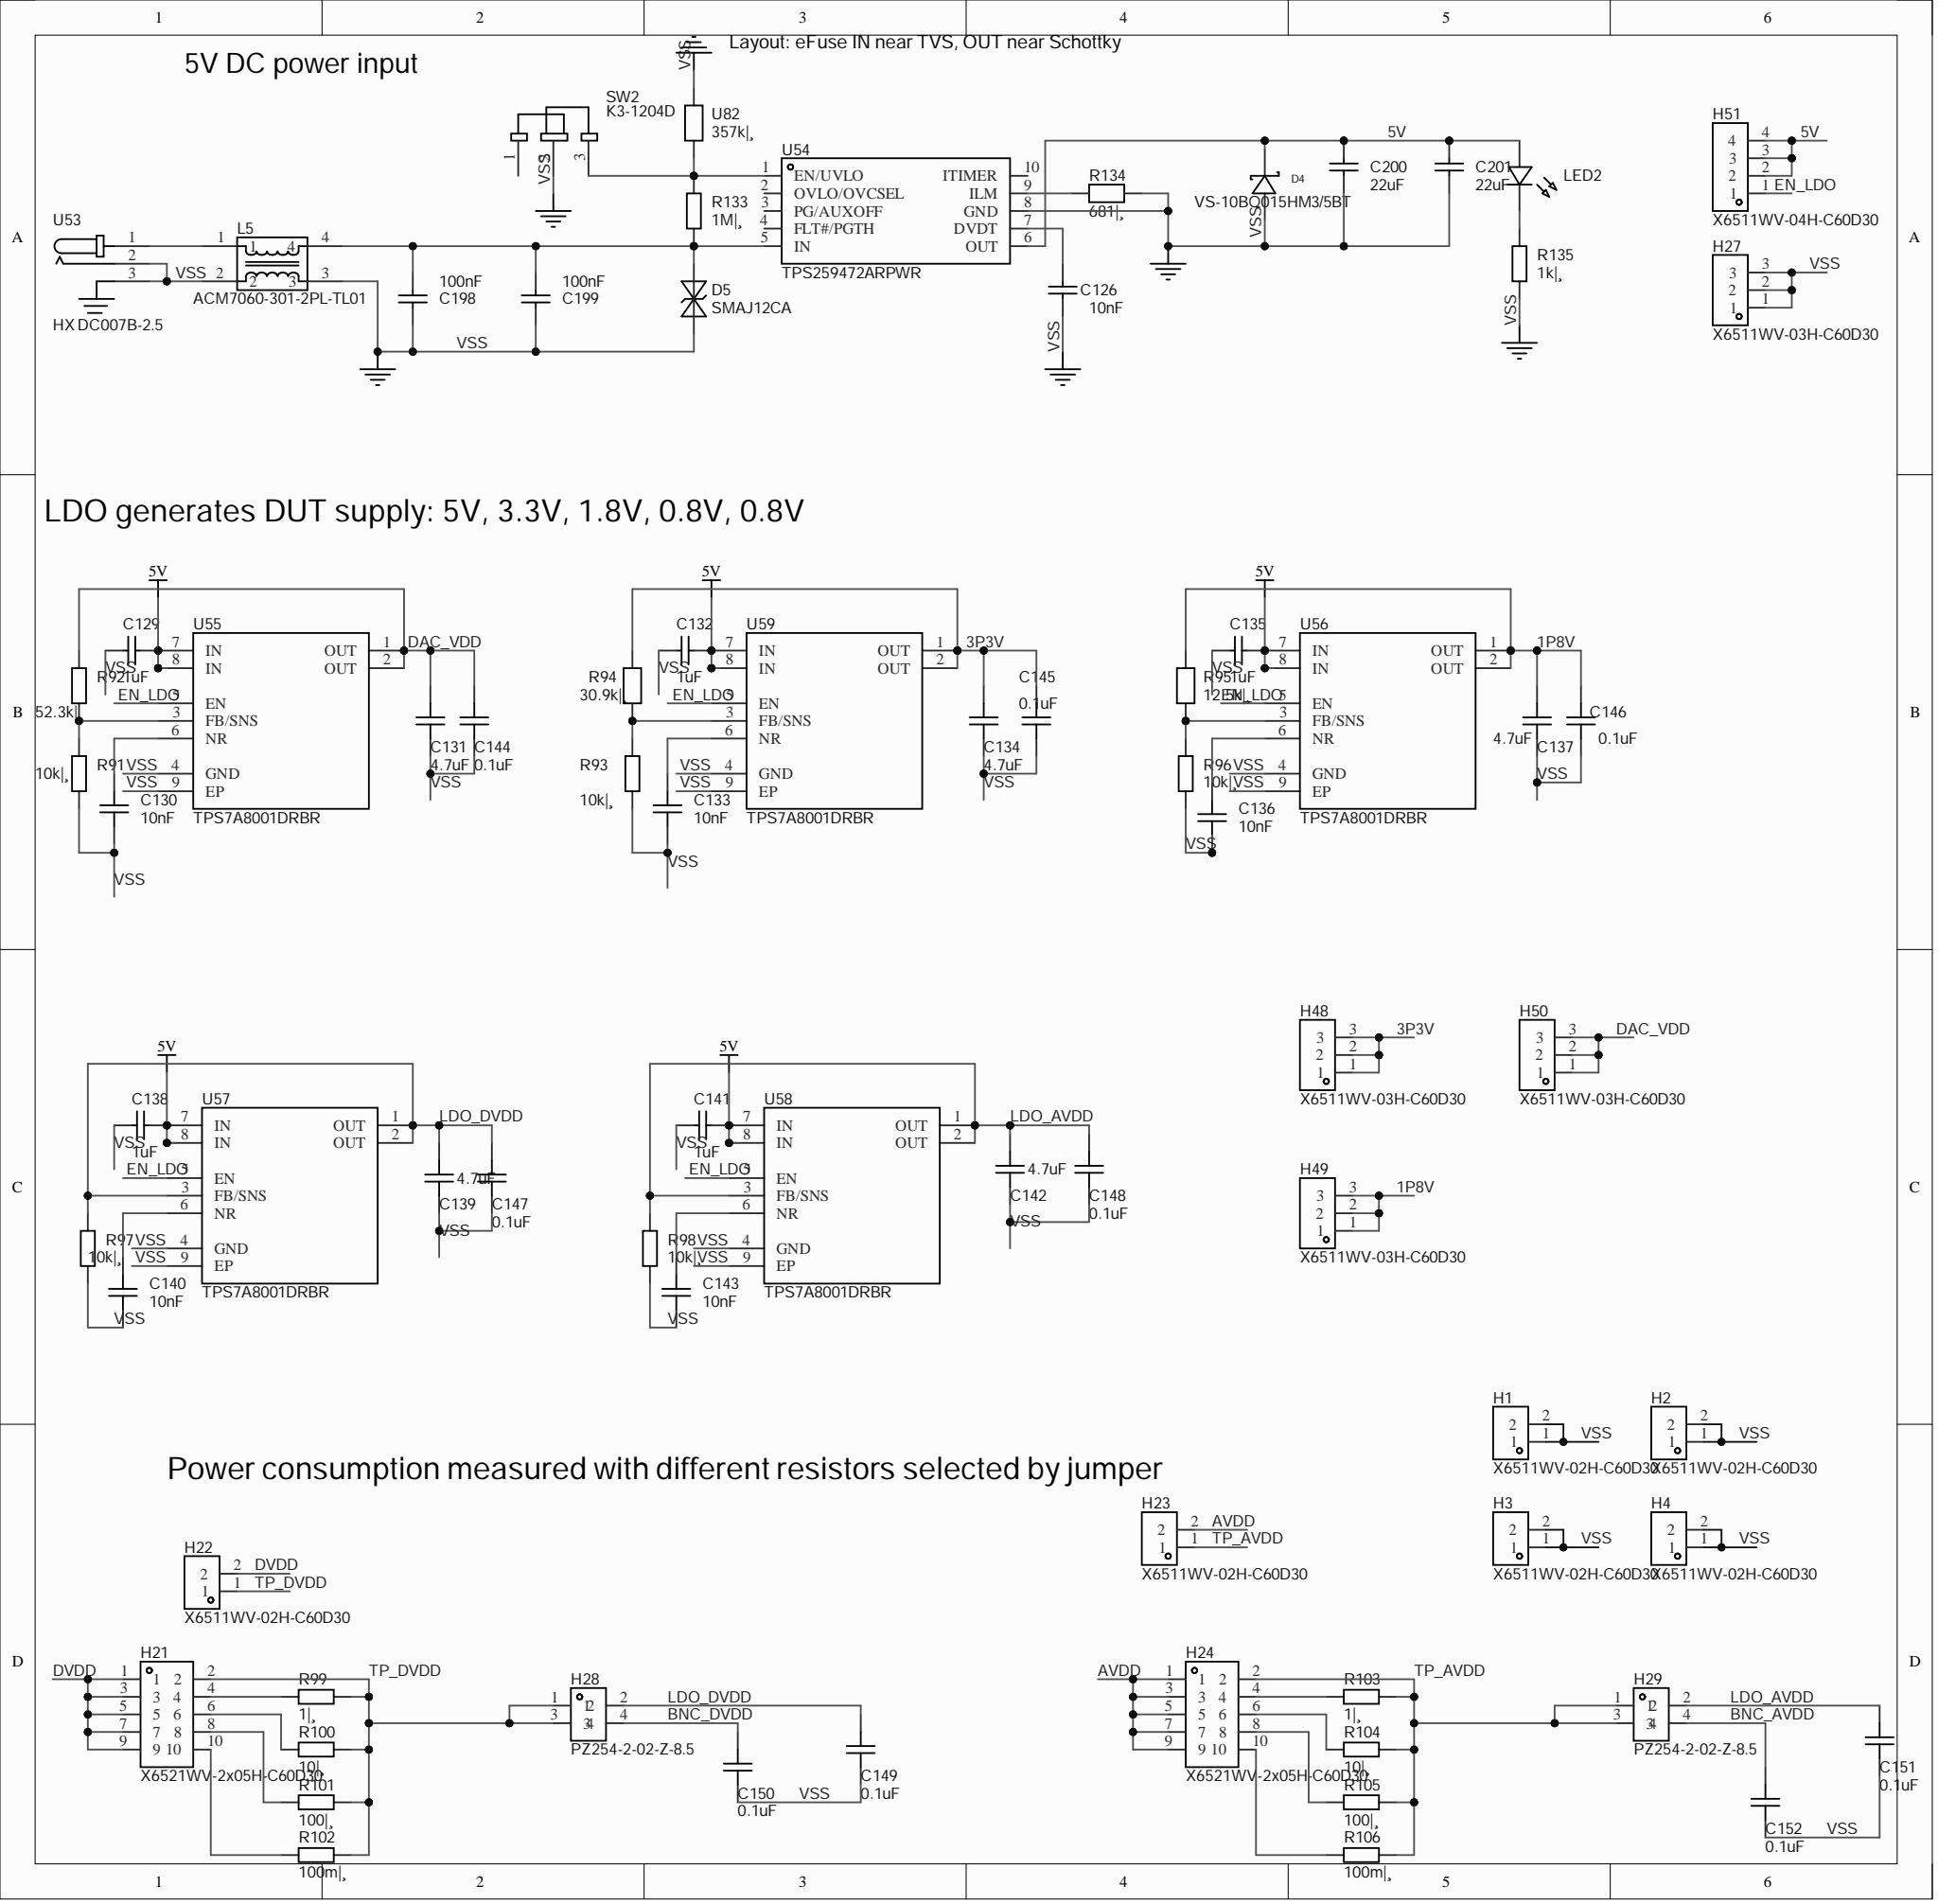Circuit board | Altium Designer | 201 parts | 197 nets | one sheet of the schematic
Parts on this sheet (reference | value | footprint):
C126 | 10nF | C0603
C129 | 1uF | C0603
C130 | 10nF | C0603
C131 | 4.7uF | C0805
C132 | 1uF | C0603
C133 | 10nF | C0603
C134 | 4.7uF | C0805
C135 | 1uF | C0603
C136 | 10nF | C0603
C137 | 4.7uF | C0805
C138 | 1uF | C0603
C139 | 4.7uF | C0805
C140 | 10nF | C0603
C141 | 1uF | C0603
C142 | 4.7uF | C0805
C143 | 10nF | C0603
C144 | 0.1uF | C0402
C145 | 0.1uF | C0402
C146 | 0.1uF | C0402
C147 | 0.1uF | C0402
C148 | 0.1uF | C0402
C149 | 0.1uF | C0402
C150 | 0.1uF | C0402
C151 | 0.1uF | C0402
C152 | 0.1uF | C0402
C198 | 100nF | C0402
C199 | 100nF | C0402
C200 | 22uF | C1206
C201 | 22uF | C1206
D4 | VS-10BQ015HM3/5BT | SMB_L4.6-W3.6-LS5.3-RD
D5 | SMAJ12CA | SMA_L4.2-W2.7-LS5.0-BI
H1 | X6511WV-02H-C60D30 | HDR-TH_2P-P2.54-V-M
H2 | X6511WV-02H-C60D30 | HDR-TH_2P-P2.54-V-M
H3 | X6511WV-02H-C60D30 | HDR-TH_2P-P2.54-V-M
H4 | X6511WV-02H-C60D30 | HDR-TH_2P-P2.54-V-M
H21 | X6521WV-2x05H-C60D30 | HDR-TH_10P-P2.54-V-M-R2-C5-S2.54
H22 | X6511WV-02H-C60D30 | HDR-TH_2P-P2.54-V-M
H23 | X6511WV-02H-C60D30 | HDR-TH_2P-P2.54-V-M
H24 | X6521WV-2x05H-C60D30 | HDR-TH_10P-P2.54-V-M-R2-C5-S2.54
H27 | X6511WV-03H-C60D30 | HDR-TH_3P-P2.54-V-M
H28 | PZ254-2-02-Z-8.5 | HDR-TH_4P-P2.54-V-M-R2-C2-S2.54
H29 | PZ254-2-02-Z-8.5 | HDR-TH_4P-P2.54-V-M-R2-C2-S2.54
H48 | X6511WV-03H-C60D30 | HDR-TH_3P-P2.54-V-M
H49 | X6511WV-03H-C60D30 | HDR-TH_3P-P2.54-V-M
H50 | X6511WV-03H-C60D30 | HDR-TH_3P-P2.54-V-M
H51 | X6511WV-04H-C60D30 | HDR-TH_4P-P2.54-V-M
L5 | ACM7060-301-2PL-TL01 | FILTER-SMD_4P-L7.0-W6.0-TL_SMCM7060
LED2 | LED_0805-R | LED_0805
R91 | 10k|¸ | R0603
R93 | 10k|¸ | R0603
R94 | 30.9k|¸ | R0603
R95 | 12.5k|¸ | R0603
R96 | 10k|¸ | R0603
R97 | 10k|¸ | R0603
R98 | 10k|¸ | R0603
R99 | 1|¸ | R1206
R100 | 10|¸ | R1206
R101 | 100|¸ | R1206
R102 | 100m|¸ | R1206
R103 | 1|¸ | R1206
R104 | 10|¸ | R1206
R105 | 100|¸ | R1206
R106 | 100m|¸ | R1206
R133 | 1M|¸ | R1206
R134 | 681|¸ | R0603
R135 | 1k|¸ | R0805
SW2 | K3-1204D | SW-TH_K3-1204D
U53 | HX DC007B-2.5 | DC-IN-TH_HX-DC007B-2.5
U54 | TPS259472ARPWR | VQFN-10_L2.0-W2.0-P0.45-TL
U55 | TPS7A8001DRBR | VSON-8_L3.0-W3.0-P0.65-TL-EP
U56 | TPS7A8001DRBR | VSON-8_L3.0-W3.0-P0.65-TL-EP
U57 | TPS7A8001DRBR | VSON-8_L3.0-W3.0-P0.65-TL-EP
U58 | TPS7A8001DRBR | VSON-8_L3.0-W3.0-P0.65-TL-EP
U59 | TPS7A8001DRBR | VSON-8_L3.0-W3.0-P0.65-TL-EP
U82 | 357k|¸ | R1206
Nets of these parts (net: part-pin ...):
VSS: C126-1 C129-1 C130-1 C131-1 C132-1 C133-1 C134-1 C135-1 C136-1 C137-1 C138-1 C139-1 C140-1 C141-1 C142-1 C143-1 C144-1 C145-1 C146-1 C147-1 C148-1 C149-1 C150-1 C151-1 C152-1 C198-1 C199-1 C200-1 C201-1 D4-2 D5-1 H1-1 H1-2 H2-1 H2-2 H3-1 H3-2 H4-1 H4-2 H27-1 H27-2 H27-3 L5-2 L5-3 R91-1 R93-1 R96-1 R97-1 R98-1 R134-2 R135-1 SW2-2 U53-2 U53-3 U54-8 U55-4 U55-9 U56-4 U56-9 U57-4 U57-9 U58-4 U58-9 U59-4 U59-9 U82-2
TP_DVDD: H21-2 H22-1 H28-1 H28-3 R99-2 R100-2 R101-2 R102-2
TP_AVDD: H23-1 H24-2 H29-1 H29-3 R103-2 R104-2 R105-2 R106-2
NetR134_1: R134-1 U54-9
NetR133_2: R133-2 SW2-3 U54-1 U82-1
NetR95_1: R95-1 R96-2 U56-3
NetR93_2: R93-2 R94-2 U59-3
NetR91_2: R91-2 U55-3
NetLED2_1: LED2-1 R135-2
NetL5_1: L5-1 U53-1
NetH24_10: H24-10 R106-1
NetH24_8: H24-8 R105-1
NetH24_6: H24-6 R104-1
NetH24_4: H24-4 R103-1
NetH21_10: H21-10 R102-1
NetH21_8: H21-8 R101-1
NetH21_6: H21-6 R100-1
NetH21_4: H21-4 R99-1
NetC198_2: C198-2 C199-2 D5-2 L5-4 R133-1 U54-5
NetC143_2: C143-2 U58-6
NetC140_2: C140-2 U57-6
NetC136_2: C136-2 U56-6
NetC133_2: C133-2 U59-6
NetC130_2: C130-2 U55-6
NetC126_2: C126-2 U54-7
LDO_DVDD: C139-2 C147-2 C149-2 H28-2 R97-2 U57-1 U57-2 U57-3
LDO_AVDD: C142-2 C148-2 C151-2 H29-2 R98-2 U58-1 U58-2 U58-3
EN_LDO: H51-1 U55-5 U56-5 U57-5 U58-5 U59-5
DVDD: H21-1 H21-3 H21-5 H21-7 H21-9 H22-2
DAC_VDD: C131-2 C144-2 H50-1 H50-2 H50-3 U55-1 U55-2
BNC_DVDD: C150-2 H28-4
BNC_AVDD: C152-2 H29-4
AVDD: H23-2 H24-1 H24-3 H24-5 H24-7 H24-9
5V: C129-2 C132-2 C135-2 C138-2 C141-2 C200-2 C201-2 D4-1 H51-2 H51-3 H51-4 LED2-2 U54-6 U55-7 U55-8 U56-7 U56-8 U57-7 U57-8 U58-7 U58-8 U59-7 U59-8
3P3V: C134-2 C145-2 H48-1 H48-2 H48-3 R94-1 U59-1 U59-2
1P8V: C137-2 C146-2 H49-1 H49-2 H49-3 R95-2 U56-1 U56-2